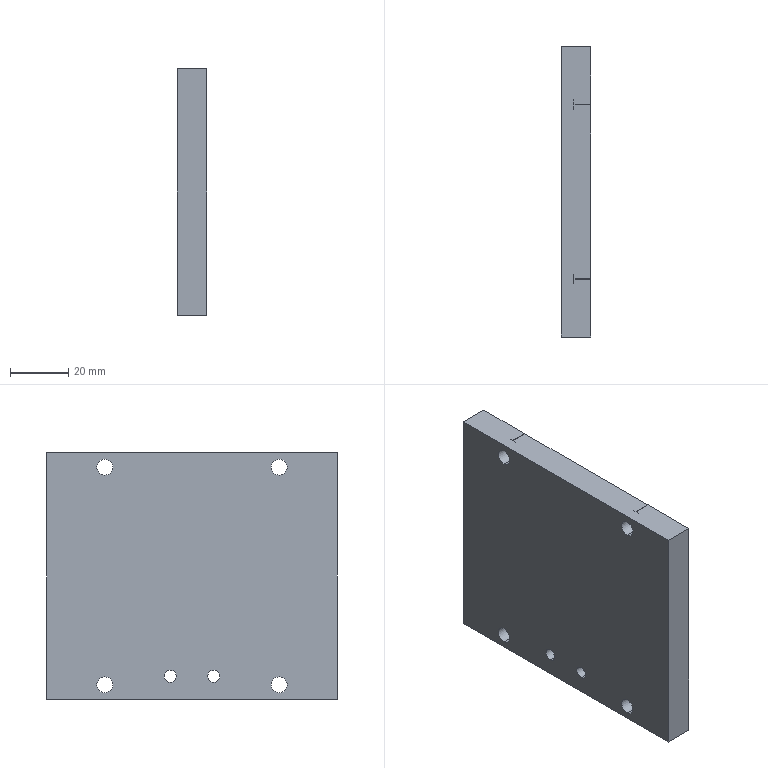Part | SolidWorks | features HoleWzd 2, Extrusion 1 | 1 solid | 28 faces | box 10 x 100 x 85 mm | volume 82523 mm3 | cylinder 18 | plane 10 | commonest cylinder face diameters 5.5 x8 10.001 x6 4.2 x4
STEP:
#1=CARTESIAN_POINT('',(0.,7.5,-32.4));
#2=VERTEX_POINT('',#1);
#3=CARTESIAN_POINT('',(0.,7.5,-36.6));
#4=VERTEX_POINT('',#3);
#5=CARTESIAN_POINT('',(0.,7.5,-34.5));
#6=DIRECTION('',(1.,0.,0.));
#7=DIRECTION('',(0.,0.,-1.));
#8=AXIS2_PLACEMENT_3D('',#5,#6,#7);
#9=CIRCLE('',#8,2.1);
#10=EDGE_CURVE('',#2,#4,#9,.T.);
#11=ORIENTED_EDGE('',*,*,#10,.F.);
#12=CARTESIAN_POINT('',(10.,7.5,-32.4));
#13=VERTEX_POINT('',#12);
#14=CARTESIAN_POINT('',(10.,7.5,-32.4));
#15=DIRECTION('',(1.,0.,0.));
#16=VECTOR('',#15,1000.);
#17=LINE('',#14,#16);
#18=EDGE_CURVE('',#2,#13,#17,.T.);
#19=ORIENTED_EDGE('',*,*,#18,.T.);
#20=CARTESIAN_POINT('',(10.,7.5,-36.6));
#21=VERTEX_POINT('',#20);
#22=CARTESIAN_POINT('',(10.,7.5,-34.5));
#23=DIRECTION('',(1.,0.,0.));
#24=DIRECTION('',(0.,0.,-1.));
#25=AXIS2_PLACEMENT_3D('',#22,#23,#24);
#26=CIRCLE('',#25,2.1);
#27=EDGE_CURVE('',#13,#21,#26,.T.);
#28=ORIENTED_EDGE('',*,*,#27,.T.);
#29=CARTESIAN_POINT('',(10.,7.5,-36.6));
#30=DIRECTION('',(1.,0.,0.));
#31=VECTOR('',#30,1000.);
#32=LINE('',#29,#31);
#33=EDGE_CURVE('',#4,#21,#32,.T.);
#34=ORIENTED_EDGE('',*,*,#33,.F.);
#35=EDGE_LOOP('',(#11,#19,#28,#34));
#36=FACE_OUTER_BOUND('',#35,.T.);
#37=CARTESIAN_POINT('',(10.,7.5,-34.5));
#38=DIRECTION('',(1.,0.,0.));
#39=DIRECTION('',(0.,0.,-1.));
#40=AXIS2_PLACEMENT_3D('',#37,#38,#39);
#41=CYLINDRICAL_SURFACE('',#40,2.1);
#42=ADVANCED_FACE('',(#36),#41,.F.);
#43=CARTESIAN_POINT('',(0.,-7.5,-32.4));
#44=VERTEX_POINT('',#43);
#45=CARTESIAN_POINT('',(0.,-7.5,-36.6));
#46=VERTEX_POINT('',#45);
#47=CARTESIAN_POINT('',(0.,-7.5,-34.5));
#48=DIRECTION('',(1.,0.,0.));
#49=DIRECTION('',(0.,0.,-1.));
#50=AXIS2_PLACEMENT_3D('',#47,#48,#49);
#51=CIRCLE('',#50,2.1);
#52=EDGE_CURVE('',#44,#46,#51,.T.);
#53=ORIENTED_EDGE('',*,*,#52,.F.);
#54=CARTESIAN_POINT('',(10.,-7.5,-32.4));
#55=VERTEX_POINT('',#54);
#56=CARTESIAN_POINT('',(10.,-7.5,-32.4));
#57=DIRECTION('',(1.,0.,0.));
#58=VECTOR('',#57,1000.);
#59=LINE('',#56,#58);
#60=EDGE_CURVE('',#44,#55,#59,.T.);
#61=ORIENTED_EDGE('',*,*,#60,.T.);
#62=CARTESIAN_POINT('',(10.,-7.5,-36.6));
#63=VERTEX_POINT('',#62);
#64=CARTESIAN_POINT('',(10.,-7.5,-34.5));
#65=DIRECTION('',(1.,0.,0.));
#66=DIRECTION('',(0.,0.,-1.));
#67=AXIS2_PLACEMENT_3D('',#64,#65,#66);
#68=CIRCLE('',#67,2.1);
#69=EDGE_CURVE('',#55,#63,#68,.T.);
#70=ORIENTED_EDGE('',*,*,#69,.T.);
#71=CARTESIAN_POINT('',(10.,-7.5,-36.6));
#72=DIRECTION('',(1.,0.,0.));
#73=VECTOR('',#72,1000.);
#74=LINE('',#71,#73);
#75=EDGE_CURVE('',#46,#63,#74,.T.);
#76=ORIENTED_EDGE('',*,*,#75,.F.);
#77=EDGE_LOOP('',(#53,#61,#70,#76));
#78=FACE_OUTER_BOUND('',#77,.T.);
#79=CARTESIAN_POINT('',(10.,-7.5,-34.5));
#80=DIRECTION('',(1.,0.,0.));
#81=DIRECTION('',(0.,0.,-1.));
#82=AXIS2_PLACEMENT_3D('',#79,#80,#81);
#83=CYLINDRICAL_SURFACE('',#82,2.1);
#84=ADVANCED_FACE('',(#78),#83,.F.);
#85=CARTESIAN_POINT('',(0.,30.,40.25));
#86=VERTEX_POINT('',#85);
#87=CARTESIAN_POINT('',(0.,30.,34.75));
#88=VERTEX_POINT('',#87);
#89=CARTESIAN_POINT('',(0.,30.,37.5));
#90=DIRECTION('',(1.,0.,0.));
#91=DIRECTION('',(0.,0.,-1.));
#92=AXIS2_PLACEMENT_3D('',#89,#90,#91);
#93=CIRCLE('',#92,2.75);
#94=EDGE_CURVE('',#86,#88,#93,.T.);
#95=ORIENTED_EDGE('',*,*,#94,.F.);
#96=CARTESIAN_POINT('',(4.3,30.,40.25));
#97=VERTEX_POINT('',#96);
#98=CARTESIAN_POINT('',(10.,30.,40.25));
#99=DIRECTION('',(1.,0.,0.));
#100=VECTOR('',#99,1000.);
#101=LINE('',#98,#100);
#102=EDGE_CURVE('',#86,#97,#101,.T.);
#103=ORIENTED_EDGE('',*,*,#102,.T.);
#104=CARTESIAN_POINT('',(4.3,30.,34.75));
#105=VERTEX_POINT('',#104);
#106=CARTESIAN_POINT('',(4.3,30.,37.5));
#107=DIRECTION('',(1.,0.,0.));
#108=DIRECTION('',(0.,0.,-1.));
#109=AXIS2_PLACEMENT_3D('',#106,#107,#108);
#110=CIRCLE('',#109,2.75);
#111=EDGE_CURVE('',#97,#105,#110,.T.);
#112=ORIENTED_EDGE('',*,*,#111,.T.);
#113=CARTESIAN_POINT('',(10.,30.,34.75));
#114=DIRECTION('',(1.,0.,0.));
#115=VECTOR('',#114,1000.);
#116=LINE('',#113,#115);
#117=EDGE_CURVE('',#88,#105,#116,.T.);
#118=ORIENTED_EDGE('',*,*,#117,.F.);
#119=EDGE_LOOP('',(#95,#103,#112,#118));
#120=FACE_OUTER_BOUND('',#119,.T.);
#121=CARTESIAN_POINT('',(10.,30.,37.5));
#122=DIRECTION('',(1.,0.,0.));
#123=DIRECTION('',(0.,0.,-1.));
#124=AXIS2_PLACEMENT_3D('',#121,#122,#123);
#125=CYLINDRICAL_SURFACE('',#124,2.75);
#126=ADVANCED_FACE('',(#120),#125,.F.);
#127=CARTESIAN_POINT('',(4.3,30.,32.499));
#128=VERTEX_POINT('',#127);
#129=CARTESIAN_POINT('',(4.3,30.071,42.5));
#130=VERTEX_POINT('',#129);
#131=CARTESIAN_POINT('',(4.3,30.,37.5));
#132=DIRECTION('',(1.,0.,0.));
#133=DIRECTION('',(0.,0.,-1.));
#134=AXIS2_PLACEMENT_3D('',#131,#132,#133);
#135=CIRCLE('',#134,5.);
#136=EDGE_CURVE('',#128,#130,#135,.T.);
#137=ORIENTED_EDGE('',*,*,#136,.F.);
#138=CARTESIAN_POINT('',(10.,30.,32.499));
#139=VERTEX_POINT('',#138);
#140=CARTESIAN_POINT('',(10.,30.,32.499));
#141=DIRECTION('',(1.,0.,0.));
#142=VECTOR('',#141,1000.);
#143=LINE('',#140,#142);
#144=EDGE_CURVE('',#128,#139,#143,.T.);
#145=ORIENTED_EDGE('',*,*,#144,.T.);
#146=CARTESIAN_POINT('',(10.,30.071,42.5));
#147=VERTEX_POINT('',#146);
#148=CARTESIAN_POINT('',(10.,30.,37.5));
#149=DIRECTION('',(1.,0.,0.));
#150=DIRECTION('',(0.,0.,-1.));
#151=AXIS2_PLACEMENT_3D('',#148,#149,#150);
#152=CIRCLE('',#151,5.);
#153=EDGE_CURVE('',#139,#147,#152,.T.);
#154=ORIENTED_EDGE('',*,*,#153,.T.);
#155=CARTESIAN_POINT('',(10.,30.071,42.5));
#156=DIRECTION('',(1.,0.,0.));
#157=VECTOR('',#156,1000.);
#158=LINE('',#155,#157);
#159=EDGE_CURVE('',#130,#147,#158,.T.);
#160=ORIENTED_EDGE('',*,*,#159,.F.);
#161=EDGE_LOOP('',(#137,#145,#154,#160));
#162=FACE_OUTER_BOUND('',#161,.T.);
#163=CARTESIAN_POINT('',(10.,30.,37.5));
#164=DIRECTION('',(1.,0.,0.));
#165=DIRECTION('',(0.,0.,-1.));
#166=AXIS2_PLACEMENT_3D('',#163,#164,#165);
#167=CYLINDRICAL_SURFACE('',#166,5.);
#168=ADVANCED_FACE('',(#162),#167,.F.);
#169=CARTESIAN_POINT('',(0.,-30.,40.25));
#170=VERTEX_POINT('',#169);
#171=CARTESIAN_POINT('',(0.,-30.,34.75));
#172=VERTEX_POINT('',#171);
#173=CARTESIAN_POINT('',(0.,-30.,37.5));
#174=DIRECTION('',(1.,0.,0.));
#175=DIRECTION('',(0.,0.,-1.));
#176=AXIS2_PLACEMENT_3D('',#173,#174,#175);
#177=CIRCLE('',#176,2.75);
#178=EDGE_CURVE('',#170,#172,#177,.T.);
#179=ORIENTED_EDGE('',*,*,#178,.F.);
#180=CARTESIAN_POINT('',(4.3,-30.,40.25));
#181=VERTEX_POINT('',#180);
#182=CARTESIAN_POINT('',(10.,-30.,40.25));
#183=DIRECTION('',(1.,0.,0.));
#184=VECTOR('',#183,1000.);
#185=LINE('',#182,#184);
#186=EDGE_CURVE('',#170,#181,#185,.T.);
#187=ORIENTED_EDGE('',*,*,#186,.T.);
#188=CARTESIAN_POINT('',(4.3,-30.,34.75));
#189=VERTEX_POINT('',#188);
#190=CARTESIAN_POINT('',(4.3,-30.,37.5));
#191=DIRECTION('',(1.,0.,0.));
#192=DIRECTION('',(0.,0.,-1.));
#193=AXIS2_PLACEMENT_3D('',#190,#191,#192);
#194=CIRCLE('',#193,2.75);
#195=EDGE_CURVE('',#181,#189,#194,.T.);
#196=ORIENTED_EDGE('',*,*,#195,.T.);
#197=CARTESIAN_POINT('',(10.,-30.,34.75));
#198=DIRECTION('',(1.,0.,0.));
#199=VECTOR('',#198,1000.);
#200=LINE('',#197,#199);
#201=EDGE_CURVE('',#172,#189,#200,.T.);
#202=ORIENTED_EDGE('',*,*,#201,.F.);
#203=EDGE_LOOP('',(#179,#187,#196,#202));
#204=FACE_OUTER_BOUND('',#203,.T.);
#205=CARTESIAN_POINT('',(10.,-30.,37.5));
#206=DIRECTION('',(1.,0.,0.));
#207=DIRECTION('',(0.,0.,-1.));
#208=AXIS2_PLACEMENT_3D('',#205,#206,#207);
#209=CYLINDRICAL_SURFACE('',#208,2.75);
#210=ADVANCED_FACE('',(#204),#209,.F.);
#211=CARTESIAN_POINT('',(4.3,-30.,32.499));
#212=VERTEX_POINT('',#211);
#213=CARTESIAN_POINT('',(4.3,-29.929,42.5));
#214=VERTEX_POINT('',#213);
#215=CARTESIAN_POINT('',(4.3,-30.,37.5));
#216=DIRECTION('',(1.,0.,0.));
#217=DIRECTION('',(0.,0.,-1.));
#218=AXIS2_PLACEMENT_3D('',#215,#216,#217);
#219=CIRCLE('',#218,5.);
#220=EDGE_CURVE('',#212,#214,#219,.T.);
#221=ORIENTED_EDGE('',*,*,#220,.F.);
#222=CARTESIAN_POINT('',(10.,-30.,32.499));
#223=VERTEX_POINT('',#222);
#224=CARTESIAN_POINT('',(10.,-30.,32.499));
#225=DIRECTION('',(1.,0.,0.));
#226=VECTOR('',#225,1000.);
#227=LINE('',#224,#226);
#228=EDGE_CURVE('',#212,#223,#227,.T.);
#229=ORIENTED_EDGE('',*,*,#228,.T.);
#230=CARTESIAN_POINT('',(10.,-29.929,42.5));
#231=VERTEX_POINT('',#230);
#232=CARTESIAN_POINT('',(10.,-30.,37.5));
#233=DIRECTION('',(1.,0.,0.));
#234=DIRECTION('',(0.,0.,-1.));
#235=AXIS2_PLACEMENT_3D('',#232,#233,#234);
#236=CIRCLE('',#235,5.);
#237=EDGE_CURVE('',#223,#231,#236,.T.);
#238=ORIENTED_EDGE('',*,*,#237,.T.);
#239=CARTESIAN_POINT('',(10.,-29.929,42.5));
#240=DIRECTION('',(1.,0.,0.));
#241=VECTOR('',#240,1000.);
#242=LINE('',#239,#241);
#243=EDGE_CURVE('',#214,#231,#242,.T.);
#244=ORIENTED_EDGE('',*,*,#243,.F.);
#245=EDGE_LOOP('',(#221,#229,#238,#244));
#246=FACE_OUTER_BOUND('',#245,.T.);
#247=CARTESIAN_POINT('',(10.,-30.,37.5));
#248=DIRECTION('',(1.,0.,0.));
#249=DIRECTION('',(0.,0.,-1.));
#250=AXIS2_PLACEMENT_3D('',#247,#248,#249);
#251=CYLINDRICAL_SURFACE('',#250,5.);
#252=ADVANCED_FACE('',(#246),#251,.F.);
#253=CARTESIAN_POINT('',(0.,30.,-34.75));
#254=VERTEX_POINT('',#253);
#255=CARTESIAN_POINT('',(0.,30.,-40.25));
#256=VERTEX_POINT('',#255);
#257=CARTESIAN_POINT('',(0.,30.,-37.5));
#258=DIRECTION('',(1.,0.,0.));
#259=DIRECTION('',(0.,0.,-1.));
#260=AXIS2_PLACEMENT_3D('',#257,#258,#259);
#261=CIRCLE('',#260,2.75);
#262=EDGE_CURVE('',#254,#256,#261,.T.);
#263=ORIENTED_EDGE('',*,*,#262,.F.);
#264=CARTESIAN_POINT('',(4.3,30.,-34.75));
#265=VERTEX_POINT('',#264);
#266=CARTESIAN_POINT('',(10.,30.,-34.75));
#267=DIRECTION('',(1.,0.,0.));
#268=VECTOR('',#267,1000.);
#269=LINE('',#266,#268);
#270=EDGE_CURVE('',#254,#265,#269,.T.);
#271=ORIENTED_EDGE('',*,*,#270,.T.);
#272=CARTESIAN_POINT('',(4.3,30.,-40.25));
#273=VERTEX_POINT('',#272);
#274=CARTESIAN_POINT('',(4.3,30.,-37.5));
#275=DIRECTION('',(1.,0.,0.));
#276=DIRECTION('',(0.,0.,-1.));
#277=AXIS2_PLACEMENT_3D('',#274,#275,#276);
#278=CIRCLE('',#277,2.75);
#279=EDGE_CURVE('',#265,#273,#278,.T.);
#280=ORIENTED_EDGE('',*,*,#279,.T.);
#281=CARTESIAN_POINT('',(10.,30.,-40.25));
#282=DIRECTION('',(1.,0.,0.));
#283=VECTOR('',#282,1000.);
#284=LINE('',#281,#283);
#285=EDGE_CURVE('',#256,#273,#284,.T.);
#286=ORIENTED_EDGE('',*,*,#285,.F.);
#287=EDGE_LOOP('',(#263,#271,#280,#286));
#288=FACE_OUTER_BOUND('',#287,.T.);
#289=CARTESIAN_POINT('',(10.,30.,-37.5));
#290=DIRECTION('',(1.,0.,0.));
#291=DIRECTION('',(0.,0.,-1.));
#292=AXIS2_PLACEMENT_3D('',#289,#290,#291);
#293=CYLINDRICAL_SURFACE('',#292,2.75);
#294=ADVANCED_FACE('',(#288),#293,.F.);
#295=CARTESIAN_POINT('',(0.,-30.,-34.75));
#296=VERTEX_POINT('',#295);
#297=CARTESIAN_POINT('',(0.,-30.,-40.25));
#298=VERTEX_POINT('',#297);
#299=CARTESIAN_POINT('',(0.,-30.,-37.5));
#300=DIRECTION('',(1.,0.,0.));
#301=DIRECTION('',(0.,0.,-1.));
#302=AXIS2_PLACEMENT_3D('',#299,#300,#301);
#303=CIRCLE('',#302,2.75);
#304=EDGE_CURVE('',#296,#298,#303,.T.);
#305=ORIENTED_EDGE('',*,*,#304,.F.);
#306=CARTESIAN_POINT('',(4.3,-30.,-34.75));
#307=VERTEX_POINT('',#306);
#308=CARTESIAN_POINT('',(10.,-30.,-34.75));
#309=DIRECTION('',(1.,0.,0.));
#310=VECTOR('',#309,1000.);
#311=LINE('',#308,#310);
#312=EDGE_CURVE('',#296,#307,#311,.T.);
#313=ORIENTED_EDGE('',*,*,#312,.T.);
#314=CARTESIAN_POINT('',(4.3,-30.,-40.25));
#315=VERTEX_POINT('',#314);
#316=CARTESIAN_POINT('',(4.3,-30.,-37.5));
#317=DIRECTION('',(1.,0.,0.));
#318=DIRECTION('',(0.,0.,-1.));
#319=AXIS2_PLACEMENT_3D('',#316,#317,#318);
#320=CIRCLE('',#319,2.75);
#321=EDGE_CURVE('',#307,#315,#320,.T.);
#322=ORIENTED_EDGE('',*,*,#321,.T.);
#323=CARTESIAN_POINT('',(10.,-30.,-40.25));
#324=DIRECTION('',(1.,0.,0.));
#325=VECTOR('',#324,1000.);
#326=LINE('',#323,#325);
#327=EDGE_CURVE('',#298,#315,#326,.T.);
#328=ORIENTED_EDGE('',*,*,#327,.F.);
#329=EDGE_LOOP('',(#305,#313,#322,#328));
#330=FACE_OUTER_BOUND('',#329,.T.);
#331=CARTESIAN_POINT('',(10.,-30.,-37.5));
#332=DIRECTION('',(1.,0.,0.));
#333=DIRECTION('',(0.,0.,-1.));
#334=AXIS2_PLACEMENT_3D('',#331,#332,#333);
#335=CYLINDRICAL_SURFACE('',#334,2.75);
#336=ADVANCED_FACE('',(#330),#335,.F.);
#337=CARTESIAN_POINT('',(4.3,30.071,-42.5));
#338=VERTEX_POINT('',#337);
#339=CARTESIAN_POINT('',(4.3,29.929,-42.5));
#340=VERTEX_POINT('',#339);
#341=CARTESIAN_POINT('',(4.3,50.,-42.5));
#342=DIRECTION('',(0.,-1.,0.));
#343=VECTOR('',#342,1000.);
#344=LINE('',#341,#343);
#345=EDGE_CURVE('',#338,#340,#344,.T.);
#346=ORIENTED_EDGE('',*,*,#345,.T.);
#347=CARTESIAN_POINT('',(10.,29.929,-42.5));
#348=VERTEX_POINT('',#347);
#349=CARTESIAN_POINT('',(10.,29.929,-42.5));
#350=DIRECTION('',(1.,0.,0.));
#351=VECTOR('',#350,1000.);
#352=LINE('',#349,#351);
#353=EDGE_CURVE('',#340,#348,#352,.T.);
#354=ORIENTED_EDGE('',*,*,#353,.T.);
#355=CARTESIAN_POINT('',(10.,-29.929,-42.5));
#356=VERTEX_POINT('',#355);
#357=CARTESIAN_POINT('',(10.,50.,-42.5));
#358=DIRECTION('',(0.,1.,0.));
#359=VECTOR('',#358,1000.);
#360=LINE('',#357,#359);
#361=EDGE_CURVE('',#356,#348,#360,.T.);
#362=ORIENTED_EDGE('',*,*,#361,.F.);
#363=CARTESIAN_POINT('',(4.3,-29.929,-42.5));
#364=VERTEX_POINT('',#363);
#365=CARTESIAN_POINT('',(10.,-29.929,-42.5));
#366=DIRECTION('',(-1.,0.,0.));
#367=VECTOR('',#366,1000.);
#368=LINE('',#365,#367);
#369=EDGE_CURVE('',#356,#364,#368,.T.);
#370=ORIENTED_EDGE('',*,*,#369,.T.);
#371=CARTESIAN_POINT('',(4.3,-30.071,-42.5));
#372=VERTEX_POINT('',#371);
#373=CARTESIAN_POINT('',(4.3,50.,-42.5));
#374=DIRECTION('',(0.,-1.,0.));
#375=VECTOR('',#374,1000.);
#376=LINE('',#373,#375);
#377=EDGE_CURVE('',#364,#372,#376,.T.);
#378=ORIENTED_EDGE('',*,*,#377,.T.);
#379=CARTESIAN_POINT('',(10.,-30.071,-42.5));
#380=VERTEX_POINT('',#379);
#381=CARTESIAN_POINT('',(10.,-30.071,-42.5));
#382=DIRECTION('',(1.,0.,0.));
#383=VECTOR('',#382,1000.);
#384=LINE('',#381,#383);
#385=EDGE_CURVE('',#372,#380,#384,.T.);
#386=ORIENTED_EDGE('',*,*,#385,.T.);
#387=CARTESIAN_POINT('',(10.,-50.,-42.5));
#388=VERTEX_POINT('',#387);
#389=CARTESIAN_POINT('',(10.,50.,-42.5));
#390=DIRECTION('',(0.,1.,0.));
#391=VECTOR('',#390,1000.);
#392=LINE('',#389,#391);
#393=EDGE_CURVE('',#388,#380,#392,.T.);
#394=ORIENTED_EDGE('',*,*,#393,.F.);
#395=CARTESIAN_POINT('',(0.,-50.,-42.5));
#396=VERTEX_POINT('',#395);
#397=CARTESIAN_POINT('',(10.,-50.,-42.5));
#398=DIRECTION('',(-1.,0.,0.));
#399=VECTOR('',#398,1000.);
#400=LINE('',#397,#399);
#401=EDGE_CURVE('',#388,#396,#400,.T.);
#402=ORIENTED_EDGE('',*,*,#401,.T.);
#403=CARTESIAN_POINT('',(0.,50.,-42.5));
#404=VERTEX_POINT('',#403);
#405=CARTESIAN_POINT('',(0.,50.,-42.5));
#406=DIRECTION('',(0.,1.,0.));
#407=VECTOR('',#406,1000.);
#408=LINE('',#405,#407);
#409=EDGE_CURVE('',#396,#404,#408,.T.);
#410=ORIENTED_EDGE('',*,*,#409,.T.);
#411=CARTESIAN_POINT('',(10.,50.,-42.5));
#412=VERTEX_POINT('',#411);
#413=CARTESIAN_POINT('',(10.,50.,-42.5));
#414=DIRECTION('',(-1.,0.,0.));
#415=VECTOR('',#414,1000.);
#416=LINE('',#413,#415);
#417=EDGE_CURVE('',#412,#404,#416,.T.);
#418=ORIENTED_EDGE('',*,*,#417,.F.);
#419=CARTESIAN_POINT('',(10.,30.071,-42.5));
#420=VERTEX_POINT('',#419);
#421=CARTESIAN_POINT('',(10.,50.,-42.5));
#422=DIRECTION('',(0.,1.,0.));
#423=VECTOR('',#422,1000.);
#424=LINE('',#421,#423);
#425=EDGE_CURVE('',#420,#412,#424,.T.);
#426=ORIENTED_EDGE('',*,*,#425,.F.);
#427=CARTESIAN_POINT('',(10.,30.071,-42.5));
#428=DIRECTION('',(-1.,0.,0.));
#429=VECTOR('',#428,1000.);
#430=LINE('',#427,#429);
#431=EDGE_CURVE('',#420,#338,#430,.T.);
#432=ORIENTED_EDGE('',*,*,#431,.T.);
#433=EDGE_LOOP('',(#346,#354,#362,#370,#378,#386,#394,#402,#410,#418,#426,#432));
#434=FACE_OUTER_BOUND('',#433,.T.);
#435=CARTESIAN_POINT('',(10.,50.,-42.5));
#436=DIRECTION('',(0.,0.,1.));
#437=DIRECTION('',(0.,-1.,0.));
#438=AXIS2_PLACEMENT_3D('',#435,#436,#437);
#439=PLANE('',#438);
#440=ADVANCED_FACE('',(#434),#439,.F.);
#441=CARTESIAN_POINT('',(0.,50.,42.5));
#442=VERTEX_POINT('',#441);
#443=CARTESIAN_POINT('',(0.,50.,42.5));
#444=DIRECTION('',(0.,0.,1.));
#445=VECTOR('',#444,1000.);
#446=LINE('',#443,#445);
#447=EDGE_CURVE('',#404,#442,#446,.T.);
#448=ORIENTED_EDGE('',*,*,#447,.T.);
#449=CARTESIAN_POINT('',(10.,50.,42.5));
#450=VERTEX_POINT('',#449);
#451=CARTESIAN_POINT('',(10.,50.,42.5));
#452=DIRECTION('',(-1.,0.,0.));
#453=VECTOR('',#452,1000.);
#454=LINE('',#451,#453);
#455=EDGE_CURVE('',#450,#442,#454,.T.);
#456=ORIENTED_EDGE('',*,*,#455,.F.);
#457=CARTESIAN_POINT('',(10.,50.,42.5));
#458=DIRECTION('',(0.,0.,1.));
#459=VECTOR('',#458,1000.);
#460=LINE('',#457,#459);
#461=EDGE_CURVE('',#412,#450,#460,.T.);
#462=ORIENTED_EDGE('',*,*,#461,.F.);
#463=ORIENTED_EDGE('',*,*,#417,.T.);
#464=EDGE_LOOP('',(#448,#456,#462,#463));
#465=FACE_OUTER_BOUND('',#464,.T.);
#466=CARTESIAN_POINT('',(10.,50.,42.5));
#467=DIRECTION('',(0.,-1.,0.));
#468=DIRECTION('',(0.,0.,-1.));
#469=AXIS2_PLACEMENT_3D('',#466,#467,#468);
#470=PLANE('',#469);
#471=ADVANCED_FACE('',(#465),#470,.F.);
#472=CARTESIAN_POINT('',(4.3,29.929,42.5));
#473=VERTEX_POINT('',#472);
#474=CARTESIAN_POINT('',(4.3,50.,42.5));
#475=DIRECTION('',(0.,1.,0.));
#476=VECTOR('',#475,1000.);
#477=LINE('',#474,#476);
#478=EDGE_CURVE('',#473,#130,#477,.T.);
#479=ORIENTED_EDGE('',*,*,#478,.T.);
#480=ORIENTED_EDGE('',*,*,#159,.T.);
#481=CARTESIAN_POINT('',(10.,50.,42.5));
#482=DIRECTION('',(0.,-1.,0.));
#483=VECTOR('',#482,1000.);
#484=LINE('',#481,#483);
#485=EDGE_CURVE('',#450,#147,#484,.T.);
#486=ORIENTED_EDGE('',*,*,#485,.F.);
#487=ORIENTED_EDGE('',*,*,#455,.T.);
#488=CARTESIAN_POINT('',(0.,-50.,42.5));
#489=VERTEX_POINT('',#488);
#490=CARTESIAN_POINT('',(0.,50.,42.5));
#491=DIRECTION('',(0.,-1.,0.));
#492=VECTOR('',#491,1000.);
#493=LINE('',#490,#492);
#494=EDGE_CURVE('',#442,#489,#493,.T.);
#495=ORIENTED_EDGE('',*,*,#494,.T.);
#496=CARTESIAN_POINT('',(10.,-50.,42.5));
#497=VERTEX_POINT('',#496);
#498=CARTESIAN_POINT('',(10.,-50.,42.5));
#499=DIRECTION('',(-1.,0.,0.));
#500=VECTOR('',#499,1000.);
#501=LINE('',#498,#500);
#502=EDGE_CURVE('',#497,#489,#501,.T.);
#503=ORIENTED_EDGE('',*,*,#502,.F.);
#504=CARTESIAN_POINT('',(10.,-30.071,42.5));
#505=VERTEX_POINT('',#504);
#506=CARTESIAN_POINT('',(10.,50.,42.5));
#507=DIRECTION('',(0.,-1.,0.));
#508=VECTOR('',#507,1000.);
#509=LINE('',#506,#508);
#510=EDGE_CURVE('',#505,#497,#509,.T.);
#511=ORIENTED_EDGE('',*,*,#510,.F.);
#512=CARTESIAN_POINT('',(4.3,-30.071,42.5));
#513=VERTEX_POINT('',#512);
#514=CARTESIAN_POINT('',(10.,-30.071,42.5));
#515=DIRECTION('',(-1.,0.,0.));
#516=VECTOR('',#515,1000.);
#517=LINE('',#514,#516);
#518=EDGE_CURVE('',#505,#513,#517,.T.);
#519=ORIENTED_EDGE('',*,*,#518,.T.);
#520=CARTESIAN_POINT('',(4.3,50.,42.5));
#521=DIRECTION('',(0.,1.,0.));
#522=VECTOR('',#521,1000.);
#523=LINE('',#520,#522);
#524=EDGE_CURVE('',#513,#214,#523,.T.);
#525=ORIENTED_EDGE('',*,*,#524,.T.);
#526=ORIENTED_EDGE('',*,*,#243,.T.);
#527=CARTESIAN_POINT('',(10.,29.929,42.5));
#528=VERTEX_POINT('',#527);
#529=CARTESIAN_POINT('',(10.,50.,42.5));
#530=DIRECTION('',(0.,-1.,0.));
#531=VECTOR('',#530,1000.);
#532=LINE('',#529,#531);
#533=EDGE_CURVE('',#528,#231,#532,.T.);
#534=ORIENTED_EDGE('',*,*,#533,.F.);
#535=CARTESIAN_POINT('',(10.,29.929,42.5));
#536=DIRECTION('',(-1.,0.,0.));
#537=VECTOR('',#536,1000.);
#538=LINE('',#535,#537);
#539=EDGE_CURVE('',#528,#473,#538,.T.);
#540=ORIENTED_EDGE('',*,*,#539,.T.);
#541=EDGE_LOOP('',(#479,#480,#486,#487,#495,#503,#511,#519,#525,#526,#534,#540));
#542=FACE_OUTER_BOUND('',#541,.T.);
#543=CARTESIAN_POINT('',(10.,50.,42.5));
#544=DIRECTION('',(0.,0.,-1.));
#545=DIRECTION('',(0.,1.,0.));
#546=AXIS2_PLACEMENT_3D('',#543,#544,#545);
#547=PLANE('',#546);
#548=ADVANCED_FACE('',(#542),#547,.F.);
#549=CARTESIAN_POINT('',(0.,-50.,42.5));
#550=DIRECTION('',(0.,0.,-1.));
#551=VECTOR('',#550,1000.);
#552=LINE('',#549,#551);
#553=EDGE_CURVE('',#489,#396,#552,.T.);
#554=ORIENTED_EDGE('',*,*,#553,.T.);
#555=ORIENTED_EDGE('',*,*,#401,.F.);
#556=CARTESIAN_POINT('',(10.,-50.,42.5));
#557=DIRECTION('',(0.,0.,-1.));
#558=VECTOR('',#557,1000.);
#559=LINE('',#556,#558);
#560=EDGE_CURVE('',#497,#388,#559,.T.);
#561=ORIENTED_EDGE('',*,*,#560,.F.);
#562=ORIENTED_EDGE('',*,*,#502,.T.);
#563=EDGE_LOOP('',(#554,#555,#561,#562));
#564=FACE_OUTER_BOUND('',#563,.T.);
#565=CARTESIAN_POINT('',(10.,-50.,42.5));
#566=DIRECTION('',(0.,1.,0.));
#567=DIRECTION('',(0.,0.,1.));
#568=AXIS2_PLACEMENT_3D('',#565,#566,#567);
#569=PLANE('',#568);
#570=ADVANCED_FACE('',(#564),#569,.F.);
#571=CARTESIAN_POINT('',(10.,7.5,-34.5));
#572=DIRECTION('',(1.,0.,0.));
#573=DIRECTION('',(0.,0.,-1.));
#574=AXIS2_PLACEMENT_3D('',#571,#572,#573);
#575=CIRCLE('',#574,2.1);
#576=EDGE_CURVE('',#21,#13,#575,.T.);
#577=ORIENTED_EDGE('',*,*,#576,.F.);
#578=ORIENTED_EDGE('',*,*,#27,.F.);
#579=EDGE_LOOP('',(#577,#578));
#580=FACE_BOUND('',#579,.T.);
#581=CARTESIAN_POINT('',(10.,-7.5,-34.5));
#582=DIRECTION('',(1.,0.,0.));
#583=DIRECTION('',(0.,0.,-1.));
#584=AXIS2_PLACEMENT_3D('',#581,#582,#583);
#585=CIRCLE('',#584,2.1);
#586=EDGE_CURVE('',#63,#55,#585,.T.);
#587=ORIENTED_EDGE('',*,*,#586,.F.);
#588=ORIENTED_EDGE('',*,*,#69,.F.);
#589=EDGE_LOOP('',(#587,#588));
#590=FACE_BOUND('',#589,.T.);
#591=CARTESIAN_POINT('',(10.,30.,37.5));
#592=DIRECTION('',(1.,0.,0.));
#593=DIRECTION('',(0.,0.,-1.));
#594=AXIS2_PLACEMENT_3D('',#591,#592,#593);
#595=CIRCLE('',#594,5.);
#596=EDGE_CURVE('',#528,#139,#595,.T.);
#597=ORIENTED_EDGE('',*,*,#596,.F.);
#598=ORIENTED_EDGE('',*,*,#533,.T.);
#599=ORIENTED_EDGE('',*,*,#237,.F.);
#600=CARTESIAN_POINT('',(10.,-30.,37.5));
#601=DIRECTION('',(1.,0.,0.));
#602=DIRECTION('',(0.,0.,-1.));
#603=AXIS2_PLACEMENT_3D('',#600,#601,#602);
#604=CIRCLE('',#603,5.);
#605=EDGE_CURVE('',#505,#223,#604,.T.);
#606=ORIENTED_EDGE('',*,*,#605,.F.);
#607=ORIENTED_EDGE('',*,*,#510,.T.);
#608=ORIENTED_EDGE('',*,*,#560,.T.);
#609=ORIENTED_EDGE('',*,*,#393,.T.);
#610=CARTESIAN_POINT('',(10.,-30.,-37.5));
#611=DIRECTION('',(1.,0.,0.));
#612=DIRECTION('',(0.,0.,-1.));
#613=AXIS2_PLACEMENT_3D('',#610,#611,#612);
#614=CIRCLE('',#613,5.);
#615=EDGE_CURVE('',#356,#380,#614,.T.);
#616=ORIENTED_EDGE('',*,*,#615,.F.);
#617=ORIENTED_EDGE('',*,*,#361,.T.);
#618=CARTESIAN_POINT('',(10.,30.,-37.5));
#619=DIRECTION('',(1.,0.,0.));
#620=DIRECTION('',(0.,0.,-1.));
#621=AXIS2_PLACEMENT_3D('',#618,#619,#620);
#622=CIRCLE('',#621,5.);
#623=EDGE_CURVE('',#420,#348,#622,.T.);
#624=ORIENTED_EDGE('',*,*,#623,.F.);
#625=ORIENTED_EDGE('',*,*,#425,.T.);
#626=ORIENTED_EDGE('',*,*,#461,.T.);
#627=ORIENTED_EDGE('',*,*,#485,.T.);
#628=ORIENTED_EDGE('',*,*,#153,.F.);
#629=EDGE_LOOP('',(#597,#598,#599,#606,#607,#608,#609,#616,#617,#624,#625,#626,#627,#628));
#630=FACE_OUTER_BOUND('',#629,.T.);
#631=CARTESIAN_POINT('',(10.,0.,0.));
#632=DIRECTION('',(1.,0.,0.));
#633=DIRECTION('',(0.,0.,-1.));
#634=AXIS2_PLACEMENT_3D('',#631,#632,#633);
#635=PLANE('',#634);
#636=ADVANCED_FACE('',(#580,#590,#630),#635,.T.);
#637=CARTESIAN_POINT('',(0.,7.5,-34.5));
#638=DIRECTION('',(1.,0.,0.));
#639=DIRECTION('',(0.,0.,-1.));
#640=AXIS2_PLACEMENT_3D('',#637,#638,#639);
#641=CIRCLE('',#640,2.1);
#642=EDGE_CURVE('',#4,#2,#641,.T.);
#643=ORIENTED_EDGE('',*,*,#642,.T.);
#644=ORIENTED_EDGE('',*,*,#10,.T.);
#645=EDGE_LOOP('',(#643,#644));
#646=FACE_BOUND('',#645,.T.);
#647=CARTESIAN_POINT('',(0.,-7.5,-34.5));
#648=DIRECTION('',(1.,0.,0.));
#649=DIRECTION('',(0.,0.,-1.));
#650=AXIS2_PLACEMENT_3D('',#647,#648,#649);
#651=CIRCLE('',#650,2.1);
#652=EDGE_CURVE('',#46,#44,#651,.T.);
#653=ORIENTED_EDGE('',*,*,#652,.T.);
#654=ORIENTED_EDGE('',*,*,#52,.T.);
#655=EDGE_LOOP('',(#653,#654));
#656=FACE_BOUND('',#655,.T.);
#657=CARTESIAN_POINT('',(0.,30.,37.5));
#658=DIRECTION('',(1.,0.,0.));
#659=DIRECTION('',(0.,0.,-1.));
#660=AXIS2_PLACEMENT_3D('',#657,#658,#659);
#661=CIRCLE('',#660,2.75);
#662=EDGE_CURVE('',#88,#86,#661,.T.);
#663=ORIENTED_EDGE('',*,*,#662,.T.);
#664=ORIENTED_EDGE('',*,*,#94,.T.);
#665=EDGE_LOOP('',(#663,#664));
#666=FACE_BOUND('',#665,.T.);
#667=CARTESIAN_POINT('',(0.,-30.,37.5));
#668=DIRECTION('',(1.,0.,0.));
#669=DIRECTION('',(0.,0.,-1.));
#670=AXIS2_PLACEMENT_3D('',#667,#668,#669);
#671=CIRCLE('',#670,2.75);
#672=EDGE_CURVE('',#172,#170,#671,.T.);
#673=ORIENTED_EDGE('',*,*,#672,.T.);
#674=ORIENTED_EDGE('',*,*,#178,.T.);
#675=EDGE_LOOP('',(#673,#674));
#676=FACE_BOUND('',#675,.T.);
#677=CARTESIAN_POINT('',(0.,30.,-37.5));
#678=DIRECTION('',(1.,0.,0.));
#679=DIRECTION('',(0.,0.,-1.));
#680=AXIS2_PLACEMENT_3D('',#677,#678,#679);
#681=CIRCLE('',#680,2.75);
#682=EDGE_CURVE('',#256,#254,#681,.T.);
#683=ORIENTED_EDGE('',*,*,#682,.T.);
#684=ORIENTED_EDGE('',*,*,#262,.T.);
#685=EDGE_LOOP('',(#683,#684));
#686=FACE_BOUND('',#685,.T.);
#687=CARTESIAN_POINT('',(0.,-30.,-37.5));
#688=DIRECTION('',(1.,0.,0.));
#689=DIRECTION('',(0.,0.,-1.));
#690=AXIS2_PLACEMENT_3D('',#687,#688,#689);
#691=CIRCLE('',#690,2.75);
#692=EDGE_CURVE('',#298,#296,#691,.T.);
#693=ORIENTED_EDGE('',*,*,#692,.T.);
#694=ORIENTED_EDGE('',*,*,#304,.T.);
#695=EDGE_LOOP('',(#693,#694));
#696=FACE_BOUND('',#695,.T.);
#697=ORIENTED_EDGE('',*,*,#409,.F.);
#698=ORIENTED_EDGE('',*,*,#553,.F.);
#699=ORIENTED_EDGE('',*,*,#494,.F.);
#700=ORIENTED_EDGE('',*,*,#447,.F.);
#701=EDGE_LOOP('',(#697,#698,#699,#700));
#702=FACE_OUTER_BOUND('',#701,.T.);
#703=CARTESIAN_POINT('',(0.,0.,0.));
#704=DIRECTION('',(1.,0.,0.));
#705=DIRECTION('',(0.,0.,-1.));
#706=AXIS2_PLACEMENT_3D('',#703,#704,#705);
#707=PLANE('',#706);
#708=ADVANCED_FACE('',(#646,#656,#666,#676,#686,#696,#702),#707,.F.);
#709=CARTESIAN_POINT('',(4.3,-30.,-37.5));
#710=DIRECTION('',(1.,0.,0.));
#711=DIRECTION('',(0.,0.,-1.));
#712=AXIS2_PLACEMENT_3D('',#709,#710,#711);
#713=CIRCLE('',#712,2.75);
#714=EDGE_CURVE('',#315,#307,#713,.T.);
#715=ORIENTED_EDGE('',*,*,#714,.F.);
#716=ORIENTED_EDGE('',*,*,#321,.F.);
#717=EDGE_LOOP('',(#715,#716));
#718=FACE_BOUND('',#717,.T.);
#719=CARTESIAN_POINT('',(4.3,-30.,-37.5));
#720=DIRECTION('',(1.,0.,0.));
#721=DIRECTION('',(0.,0.,-1.));
#722=AXIS2_PLACEMENT_3D('',#719,#720,#721);
#723=CIRCLE('',#722,5.);
#724=EDGE_CURVE('',#364,#372,#723,.T.);
#725=ORIENTED_EDGE('',*,*,#724,.T.);
#726=ORIENTED_EDGE('',*,*,#377,.F.);
#727=EDGE_LOOP('',(#725,#726));
#728=FACE_OUTER_BOUND('',#727,.T.);
#729=CARTESIAN_POINT('',(4.3,-27.25,-37.5));
#730=DIRECTION('',(-1.,0.,0.));
#731=DIRECTION('',(0.,0.,1.));
#732=AXIS2_PLACEMENT_3D('',#729,#730,#731);
#733=PLANE('',#732);
#734=ADVANCED_FACE('',(#718,#728),#733,.F.);
#735=ORIENTED_EDGE('',*,*,#724,.F.);
#736=ORIENTED_EDGE('',*,*,#369,.F.);
#737=ORIENTED_EDGE('',*,*,#615,.T.);
#738=ORIENTED_EDGE('',*,*,#385,.F.);
#739=EDGE_LOOP('',(#735,#736,#737,#738));
#740=FACE_OUTER_BOUND('',#739,.T.);
#741=CARTESIAN_POINT('',(10.,-30.,-37.5));
#742=DIRECTION('',(1.,0.,0.));
#743=DIRECTION('',(0.,0.,-1.));
#744=AXIS2_PLACEMENT_3D('',#741,#742,#743);
#745=CYLINDRICAL_SURFACE('',#744,5.);
#746=ADVANCED_FACE('',(#740),#745,.F.);
#747=ORIENTED_EDGE('',*,*,#312,.F.);
#748=ORIENTED_EDGE('',*,*,#692,.F.);
#749=ORIENTED_EDGE('',*,*,#327,.T.);
#750=ORIENTED_EDGE('',*,*,#714,.T.);
#751=EDGE_LOOP('',(#747,#748,#749,#750));
#752=FACE_OUTER_BOUND('',#751,.T.);
#753=CARTESIAN_POINT('',(10.,-30.,-37.5));
#754=DIRECTION('',(1.,0.,0.));
#755=DIRECTION('',(0.,0.,-1.));
#756=AXIS2_PLACEMENT_3D('',#753,#754,#755);
#757=CYLINDRICAL_SURFACE('',#756,2.75);
#758=ADVANCED_FACE('',(#752),#757,.F.);
#759=CARTESIAN_POINT('',(4.3,30.,-37.5));
#760=DIRECTION('',(1.,0.,0.));
#761=DIRECTION('',(0.,0.,-1.));
#762=AXIS2_PLACEMENT_3D('',#759,#760,#761);
#763=CIRCLE('',#762,2.75);
#764=EDGE_CURVE('',#273,#265,#763,.T.);
#765=ORIENTED_EDGE('',*,*,#764,.F.);
#766=ORIENTED_EDGE('',*,*,#279,.F.);
#767=EDGE_LOOP('',(#765,#766));
#768=FACE_BOUND('',#767,.T.);
#769=CARTESIAN_POINT('',(4.3,30.,-37.5));
#770=DIRECTION('',(1.,0.,0.));
#771=DIRECTION('',(0.,0.,-1.));
#772=AXIS2_PLACEMENT_3D('',#769,#770,#771);
#773=CIRCLE('',#772,5.);
#774=EDGE_CURVE('',#338,#340,#773,.T.);
#775=ORIENTED_EDGE('',*,*,#774,.T.);
#776=ORIENTED_EDGE('',*,*,#345,.F.);
#777=EDGE_LOOP('',(#775,#776));
#778=FACE_OUTER_BOUND('',#777,.T.);
#779=CARTESIAN_POINT('',(4.3,32.75,-37.5));
#780=DIRECTION('',(-1.,0.,0.));
#781=DIRECTION('',(0.,0.,1.));
#782=AXIS2_PLACEMENT_3D('',#779,#780,#781);
#783=PLANE('',#782);
#784=ADVANCED_FACE('',(#768,#778),#783,.F.);
#785=ORIENTED_EDGE('',*,*,#774,.F.);
#786=ORIENTED_EDGE('',*,*,#431,.F.);
#787=ORIENTED_EDGE('',*,*,#623,.T.);
#788=ORIENTED_EDGE('',*,*,#353,.F.);
#789=EDGE_LOOP('',(#785,#786,#787,#788));
#790=FACE_OUTER_BOUND('',#789,.T.);
#791=CARTESIAN_POINT('',(10.,30.,-37.5));
#792=DIRECTION('',(1.,0.,0.));
#793=DIRECTION('',(0.,0.,-1.));
#794=AXIS2_PLACEMENT_3D('',#791,#792,#793);
#795=CYLINDRICAL_SURFACE('',#794,5.);
#796=ADVANCED_FACE('',(#790),#795,.F.);
#797=ORIENTED_EDGE('',*,*,#270,.F.);
#798=ORIENTED_EDGE('',*,*,#682,.F.);
#799=ORIENTED_EDGE('',*,*,#285,.T.);
#800=ORIENTED_EDGE('',*,*,#764,.T.);
#801=EDGE_LOOP('',(#797,#798,#799,#800));
#802=FACE_OUTER_BOUND('',#801,.T.);
#803=CARTESIAN_POINT('',(10.,30.,-37.5));
#804=DIRECTION('',(1.,0.,0.));
#805=DIRECTION('',(0.,0.,-1.));
#806=AXIS2_PLACEMENT_3D('',#803,#804,#805);
#807=CYLINDRICAL_SURFACE('',#806,2.75);
#808=ADVANCED_FACE('',(#802),#807,.F.);
#809=CARTESIAN_POINT('',(4.3,-30.,37.5));
#810=DIRECTION('',(1.,0.,0.));
#811=DIRECTION('',(0.,0.,-1.));
#812=AXIS2_PLACEMENT_3D('',#809,#810,#811);
#813=CIRCLE('',#812,2.75);
#814=EDGE_CURVE('',#189,#181,#813,.T.);
#815=ORIENTED_EDGE('',*,*,#814,.F.);
#816=ORIENTED_EDGE('',*,*,#195,.F.);
#817=EDGE_LOOP('',(#815,#816));
#818=FACE_BOUND('',#817,.T.);
#819=CARTESIAN_POINT('',(4.3,-30.,37.5));
#820=DIRECTION('',(1.,0.,0.));
#821=DIRECTION('',(0.,0.,-1.));
#822=AXIS2_PLACEMENT_3D('',#819,#820,#821);
#823=CIRCLE('',#822,5.);
#824=EDGE_CURVE('',#513,#212,#823,.T.);
#825=ORIENTED_EDGE('',*,*,#824,.T.);
#826=ORIENTED_EDGE('',*,*,#220,.T.);
#827=ORIENTED_EDGE('',*,*,#524,.F.);
#828=EDGE_LOOP('',(#825,#826,#827));
#829=FACE_OUTER_BOUND('',#828,.T.);
#830=CARTESIAN_POINT('',(4.3,-27.25,37.5));
#831=DIRECTION('',(-1.,0.,0.));
#832=DIRECTION('',(0.,0.,1.));
#833=AXIS2_PLACEMENT_3D('',#830,#831,#832);
#834=PLANE('',#833);
#835=ADVANCED_FACE('',(#818,#829),#834,.F.);
#836=ORIENTED_EDGE('',*,*,#228,.F.);
#837=ORIENTED_EDGE('',*,*,#824,.F.);
#838=ORIENTED_EDGE('',*,*,#518,.F.);
#839=ORIENTED_EDGE('',*,*,#605,.T.);
#840=EDGE_LOOP('',(#836,#837,#838,#839));
#841=FACE_OUTER_BOUND('',#840,.T.);
#842=CARTESIAN_POINT('',(10.,-30.,37.5));
#843=DIRECTION('',(1.,0.,0.));
#844=DIRECTION('',(0.,0.,-1.));
#845=AXIS2_PLACEMENT_3D('',#842,#843,#844);
#846=CYLINDRICAL_SURFACE('',#845,5.);
#847=ADVANCED_FACE('',(#841),#846,.F.);
#848=ORIENTED_EDGE('',*,*,#186,.F.);
#849=ORIENTED_EDGE('',*,*,#672,.F.);
#850=ORIENTED_EDGE('',*,*,#201,.T.);
#851=ORIENTED_EDGE('',*,*,#814,.T.);
#852=EDGE_LOOP('',(#848,#849,#850,#851));
#853=FACE_OUTER_BOUND('',#852,.T.);
#854=CARTESIAN_POINT('',(10.,-30.,37.5));
#855=DIRECTION('',(1.,0.,0.));
#856=DIRECTION('',(0.,0.,-1.));
#857=AXIS2_PLACEMENT_3D('',#854,#855,#856);
#858=CYLINDRICAL_SURFACE('',#857,2.75);
#859=ADVANCED_FACE('',(#853),#858,.F.);
#860=CARTESIAN_POINT('',(4.3,30.,37.5));
#861=DIRECTION('',(1.,0.,0.));
#862=DIRECTION('',(0.,0.,-1.));
#863=AXIS2_PLACEMENT_3D('',#860,#861,#862);
#864=CIRCLE('',#863,2.75);
#865=EDGE_CURVE('',#105,#97,#864,.T.);
#866=ORIENTED_EDGE('',*,*,#865,.F.);
#867=ORIENTED_EDGE('',*,*,#111,.F.);
#868=EDGE_LOOP('',(#866,#867));
#869=FACE_BOUND('',#868,.T.);
#870=CARTESIAN_POINT('',(4.3,30.,37.5));
#871=DIRECTION('',(1.,0.,0.));
#872=DIRECTION('',(0.,0.,-1.));
#873=AXIS2_PLACEMENT_3D('',#870,#871,#872);
#874=CIRCLE('',#873,5.);
#875=EDGE_CURVE('',#473,#128,#874,.T.);
#876=ORIENTED_EDGE('',*,*,#875,.T.);
#877=ORIENTED_EDGE('',*,*,#136,.T.);
#878=ORIENTED_EDGE('',*,*,#478,.F.);
#879=EDGE_LOOP('',(#876,#877,#878));
#880=FACE_OUTER_BOUND('',#879,.T.);
#881=CARTESIAN_POINT('',(4.3,32.75,37.5));
#882=DIRECTION('',(-1.,0.,0.));
#883=DIRECTION('',(0.,0.,1.));
#884=AXIS2_PLACEMENT_3D('',#881,#882,#883);
#885=PLANE('',#884);
#886=ADVANCED_FACE('',(#869,#880),#885,.F.);
#887=ORIENTED_EDGE('',*,*,#144,.F.);
#888=ORIENTED_EDGE('',*,*,#875,.F.);
#889=ORIENTED_EDGE('',*,*,#539,.F.);
#890=ORIENTED_EDGE('',*,*,#596,.T.);
#891=EDGE_LOOP('',(#887,#888,#889,#890));
#892=FACE_OUTER_BOUND('',#891,.T.);
#893=CARTESIAN_POINT('',(10.,30.,37.5));
#894=DIRECTION('',(1.,0.,0.));
#895=DIRECTION('',(0.,0.,-1.));
#896=AXIS2_PLACEMENT_3D('',#893,#894,#895);
#897=CYLINDRICAL_SURFACE('',#896,5.);
#898=ADVANCED_FACE('',(#892),#897,.F.);
#899=ORIENTED_EDGE('',*,*,#102,.F.);
#900=ORIENTED_EDGE('',*,*,#662,.F.);
#901=ORIENTED_EDGE('',*,*,#117,.T.);
#902=ORIENTED_EDGE('',*,*,#865,.T.);
#903=EDGE_LOOP('',(#899,#900,#901,#902));
#904=FACE_OUTER_BOUND('',#903,.T.);
#905=CARTESIAN_POINT('',(10.,30.,37.5));
#906=DIRECTION('',(1.,0.,0.));
#907=DIRECTION('',(0.,0.,-1.));
#908=AXIS2_PLACEMENT_3D('',#905,#906,#907);
#909=CYLINDRICAL_SURFACE('',#908,2.75);
#910=ADVANCED_FACE('',(#904),#909,.F.);
#911=ORIENTED_EDGE('',*,*,#60,.F.);
#912=ORIENTED_EDGE('',*,*,#652,.F.);
#913=ORIENTED_EDGE('',*,*,#75,.T.);
#914=ORIENTED_EDGE('',*,*,#586,.T.);
#915=EDGE_LOOP('',(#911,#912,#913,#914));
#916=FACE_OUTER_BOUND('',#915,.T.);
#917=CARTESIAN_POINT('',(10.,-7.5,-34.5));
#918=DIRECTION('',(1.,0.,0.));
#919=DIRECTION('',(0.,0.,-1.));
#920=AXIS2_PLACEMENT_3D('',#917,#918,#919);
#921=CYLINDRICAL_SURFACE('',#920,2.1);
#922=ADVANCED_FACE('',(#916),#921,.F.);
#923=ORIENTED_EDGE('',*,*,#18,.F.);
#924=ORIENTED_EDGE('',*,*,#642,.F.);
#925=ORIENTED_EDGE('',*,*,#33,.T.);
#926=ORIENTED_EDGE('',*,*,#576,.T.);
#927=EDGE_LOOP('',(#923,#924,#925,#926));
#928=FACE_OUTER_BOUND('',#927,.T.);
#929=CARTESIAN_POINT('',(10.,7.5,-34.5));
#930=DIRECTION('',(1.,0.,0.));
#931=DIRECTION('',(0.,0.,-1.));
#932=AXIS2_PLACEMENT_3D('',#929,#930,#931);
#933=CYLINDRICAL_SURFACE('',#932,2.1);
#934=ADVANCED_FACE('',(#928),#933,.F.);
#935=CLOSED_SHELL('',(#42,#84,#126,#168,#210,#252,#294,#336,#440,#471,#548,#570,#636,#708,#734,#746,#758,#784,#796,#808,#835,#847,#859,#886,#898,#910,#922,#934));
#936=MANIFOLD_SOLID_BREP('',#935);
#937=CARTESIAN_POINT('',(0.,0.,0.));
#938=DIRECTION('',(0.,0.,1.));
#939=DIRECTION('',(1.,0.,0.));
#940=AXIS2_PLACEMENT_3D('',#937,#938,#939);
#941=(LENGTH_UNIT()NAMED_UNIT(*)SI_UNIT(.MILLI.,.METRE.));
#942=UNCERTAINTY_MEASURE_WITH_UNIT(LENGTH_MEASURE(0.00001),#941,'','');
#943=(NAMED_UNIT(*)PLANE_ANGLE_UNIT()SI_UNIT($,.RADIAN.));
#944=(NAMED_UNIT(*)SI_UNIT($,.STERADIAN.)SOLID_ANGLE_UNIT());
#945=(GEOMETRIC_REPRESENTATION_CONTEXT(3)GLOBAL_UNCERTAINTY_ASSIGNED_CONTEXT((#942))GLOBAL_UNIT_ASSIGNED_CONTEXT((#941,#943,#944))REPRESENTATION_CONTEXT('',''));
#946=ADVANCED_BREP_SHAPE_REPRESENTATION('',(#936,#940),#945);